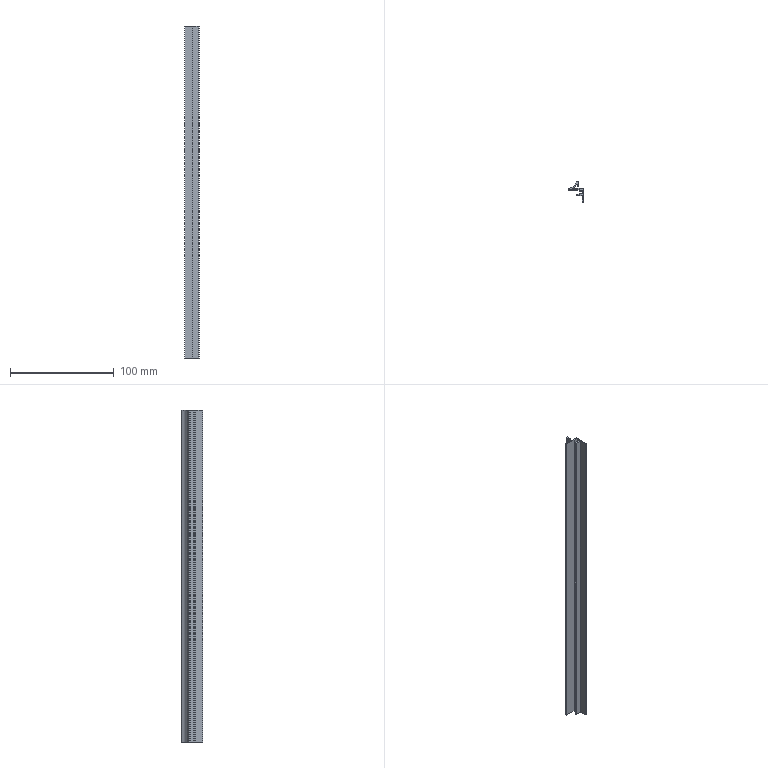Part | SolidWorks | features BaseBody 1, ICE 1, MoveFace 1 | 1 solid | 27 faces | box 14 x 20.3 x 320 mm | volume 16293 mm3 | plane 20 | cylinder 7 | commonest cylinder face diameters 0.387 x2 0.8 x2 0.4 x1 20 x1 22 x1
STEP:
#1=CARTESIAN_POINT('',(-5.304,-0.625,200.));
#2=VERTEX_POINT('',#1);
#3=CARTESIAN_POINT('',(-5.449,-0.8125,200.));
#4=VERTEX_POINT('',#3);
#5=CARTESIAN_POINT('',(-5.255,-0.8125,200.));
#6=DIRECTION('',(0.,0.,1.));
#7=DIRECTION('',(-1.,0.,0.));
#8=AXIS2_PLACEMENT_3D('',#5,#6,#7);
#9=CIRCLE('',#8,0.1937);
#10=EDGE_CURVE('',#2,#4,#9,.T.);
#11=ORIENTED_EDGE('',*,*,#10,.T.);
#12=CARTESIAN_POINT('',(-5.449,-0.8125,-120.));
#13=VERTEX_POINT('',#12);
#14=CARTESIAN_POINT('',(-5.449,-0.8125,230.));
#15=DIRECTION('',(0.,0.,-1.));
#16=VECTOR('',#15,1000.);
#17=LINE('',#14,#16);
#18=EDGE_CURVE('',#4,#13,#17,.T.);
#19=ORIENTED_EDGE('',*,*,#18,.T.);
#20=CARTESIAN_POINT('',(-5.304,-0.625,-120.));
#21=VERTEX_POINT('',#20);
#22=CARTESIAN_POINT('',(-5.255,-0.8125,-120.));
#23=DIRECTION('',(0.,0.,-1.));
#24=DIRECTION('',(1.,0.,0.));
#25=AXIS2_PLACEMENT_3D('',#22,#23,#24);
#26=CIRCLE('',#25,0.1937);
#27=EDGE_CURVE('',#13,#21,#26,.T.);
#28=ORIENTED_EDGE('',*,*,#27,.T.);
#29=CARTESIAN_POINT('',(-5.304,-0.625,230.));
#30=DIRECTION('',(0.,0.,-1.));
#31=VECTOR('',#30,1000.);
#32=LINE('',#29,#31);
#33=EDGE_CURVE('',#2,#21,#32,.T.);
#34=ORIENTED_EDGE('',*,*,#33,.F.);
#35=EDGE_LOOP('',(#11,#19,#28,#34));
#36=FACE_OUTER_BOUND('',#35,.T.);
#37=CARTESIAN_POINT('',(-5.255,-0.8125,230.));
#38=DIRECTION('',(0.,0.,-1.));
#39=DIRECTION('',(-1.,0.,0.));
#40=AXIS2_PLACEMENT_3D('',#37,#38,#39);
#41=CYLINDRICAL_SURFACE('',#40,0.1937);
#42=ADVANCED_FACE('',(#36),#41,.F.);
#43=CARTESIAN_POINT('',(5.,-1.,-120.));
#44=VERTEX_POINT('',#43);
#45=CARTESIAN_POINT('',(5.,-14.3,-120.));
#46=VERTEX_POINT('',#45);
#47=CARTESIAN_POINT('',(5.,29.623,-120.));
#48=DIRECTION('',(0.,-1.,0.));
#49=VECTOR('',#48,1000.);
#50=LINE('',#47,#49);
#51=EDGE_CURVE('',#44,#46,#50,.T.);
#52=ORIENTED_EDGE('',*,*,#51,.F.);
#53=CARTESIAN_POINT('',(5.,-1.,200.));
#54=VERTEX_POINT('',#53);
#55=CARTESIAN_POINT('',(5.,-1.,230.));
#56=DIRECTION('',(0.,0.,-1.));
#57=VECTOR('',#56,1000.);
#58=LINE('',#55,#57);
#59=EDGE_CURVE('',#54,#44,#58,.T.);
#60=ORIENTED_EDGE('',*,*,#59,.F.);
#61=CARTESIAN_POINT('',(5.,-14.3,200.));
#62=VERTEX_POINT('',#61);
#63=CARTESIAN_POINT('',(5.,-14.3,200.));
#64=DIRECTION('',(0.,1.,0.));
#65=VECTOR('',#64,1000.);
#66=LINE('',#63,#65);
#67=EDGE_CURVE('',#62,#54,#66,.T.);
#68=ORIENTED_EDGE('',*,*,#67,.F.);
#69=CARTESIAN_POINT('',(5.,-14.3,230.));
#70=DIRECTION('',(0.,0.,1.));
#71=VECTOR('',#70,1000.);
#72=LINE('',#69,#71);
#73=EDGE_CURVE('',#46,#62,#72,.T.);
#74=ORIENTED_EDGE('',*,*,#73,.F.);
#75=EDGE_LOOP('',(#52,#60,#68,#74));
#76=FACE_OUTER_BOUND('',#75,.T.);
#77=CARTESIAN_POINT('',(5.,-14.3,230.));
#78=DIRECTION('',(-1.,0.,0.));
#79=DIRECTION('',(0.,0.,1.));
#80=AXIS2_PLACEMENT_3D('',#77,#78,#79);
#81=PLANE('',#80);
#82=ADVANCED_FACE('',(#76),#81,.F.);
#83=CARTESIAN_POINT('',(-9.,-2.,-120.));
#84=VERTEX_POINT('',#83);
#85=CARTESIAN_POINT('',(-9.,-2.,200.));
#86=VERTEX_POINT('',#85);
#87=CARTESIAN_POINT('',(-9.,-2.,230.));
#88=DIRECTION('',(0.,0.,1.));
#89=VECTOR('',#88,1000.);
#90=LINE('',#87,#89);
#91=EDGE_CURVE('',#84,#86,#90,.T.);
#92=ORIENTED_EDGE('',*,*,#91,.F.);
#93=CARTESIAN_POINT('',(0.9,-2.,-120.));
#94=VERTEX_POINT('',#93);
#95=CARTESIAN_POINT('',(5.,-2.,-120.));
#96=DIRECTION('',(-1.,0.,0.));
#97=VECTOR('',#96,1000.);
#98=LINE('',#95,#97);
#99=EDGE_CURVE('',#94,#84,#98,.T.);
#100=ORIENTED_EDGE('',*,*,#99,.F.);
#101=CARTESIAN_POINT('',(0.9,-2.,200.));
#102=VERTEX_POINT('',#101);
#103=CARTESIAN_POINT('',(0.9,-2.,230.));
#104=DIRECTION('',(0.,0.,-1.));
#105=VECTOR('',#104,1000.);
#106=LINE('',#103,#105);
#107=EDGE_CURVE('',#102,#94,#106,.T.);
#108=ORIENTED_EDGE('',*,*,#107,.F.);
#109=CARTESIAN_POINT('',(5.,-2.,200.));
#110=DIRECTION('',(1.,0.,0.));
#111=VECTOR('',#110,1000.);
#112=LINE('',#109,#111);
#113=EDGE_CURVE('',#86,#102,#112,.T.);
#114=ORIENTED_EDGE('',*,*,#113,.F.);
#115=EDGE_LOOP('',(#92,#100,#108,#114));
#116=FACE_OUTER_BOUND('',#115,.T.);
#117=CARTESIAN_POINT('',(-9.,-2.,230.));
#118=DIRECTION('',(0.,1.,0.));
#119=DIRECTION('',(0.,0.,1.));
#120=AXIS2_PLACEMENT_3D('',#117,#118,#119);
#121=PLANE('',#120);
#122=ADVANCED_FACE('',(#116),#121,.F.);
#123=CARTESIAN_POINT('',(4.,-6.,200.));
#124=VERTEX_POINT('',#123);
#125=CARTESIAN_POINT('',(4.,-3.,200.));
#126=VERTEX_POINT('',#125);
#127=CARTESIAN_POINT('',(4.,29.623,200.));
#128=DIRECTION('',(0.,1.,0.));
#129=VECTOR('',#128,1000.);
#130=LINE('',#127,#129);
#131=EDGE_CURVE('',#124,#126,#130,.T.);
#132=ORIENTED_EDGE('',*,*,#131,.F.);
#133=CARTESIAN_POINT('',(1.,-6.,200.));
#134=VERTEX_POINT('',#133);
#135=CARTESIAN_POINT('',(5.,-6.,200.));
#136=DIRECTION('',(1.,0.,0.));
#137=VECTOR('',#136,1000.);
#138=LINE('',#135,#137);
#139=EDGE_CURVE('',#134,#124,#138,.T.);
#140=ORIENTED_EDGE('',*,*,#139,.F.);
#141=CARTESIAN_POINT('',(1.,-6.7,200.));
#142=VERTEX_POINT('',#141);
#143=CARTESIAN_POINT('',(1.,-6.,200.));
#144=DIRECTION('',(0.,-1.,0.));
#145=VECTOR('',#144,1000.);
#146=LINE('',#143,#145);
#147=EDGE_CURVE('',#134,#142,#146,.T.);
#148=ORIENTED_EDGE('',*,*,#147,.T.);
#149=CARTESIAN_POINT('',(-1.7,-6.7,200.));
#150=VERTEX_POINT('',#149);
#151=CARTESIAN_POINT('',(5.,-6.7,200.));
#152=DIRECTION('',(1.,0.,0.));
#153=VECTOR('',#152,1000.);
#154=LINE('',#151,#153);
#155=EDGE_CURVE('',#150,#142,#154,.T.);
#156=ORIENTED_EDGE('',*,*,#155,.F.);
#157=CARTESIAN_POINT('',(-1.7,-7.7,200.));
#158=VERTEX_POINT('',#157);
#159=CARTESIAN_POINT('',(-1.7,-6.7,200.));
#160=DIRECTION('',(0.,-1.,0.));
#161=VECTOR('',#160,1000.);
#162=LINE('',#159,#161);
#163=EDGE_CURVE('',#150,#158,#162,.T.);
#164=ORIENTED_EDGE('',*,*,#163,.T.);
#165=CARTESIAN_POINT('',(4.,-7.7,200.));
#166=VERTEX_POINT('',#165);
#167=CARTESIAN_POINT('',(5.,-7.7,200.));
#168=DIRECTION('',(-1.,0.,0.));
#169=VECTOR('',#168,1000.);
#170=LINE('',#167,#169);
#171=EDGE_CURVE('',#166,#158,#170,.T.);
#172=ORIENTED_EDGE('',*,*,#171,.F.);
#173=CARTESIAN_POINT('',(4.,-14.3,200.));
#174=VERTEX_POINT('',#173);
#175=CARTESIAN_POINT('',(4.,29.623,200.));
#176=DIRECTION('',(0.,1.,0.));
#177=VECTOR('',#176,1000.);
#178=LINE('',#175,#177);
#179=EDGE_CURVE('',#174,#166,#178,.T.);
#180=ORIENTED_EDGE('',*,*,#179,.F.);
#181=CARTESIAN_POINT('',(5.,-14.3,200.));
#182=DIRECTION('',(-1.,0.,0.));
#183=VECTOR('',#182,1000.);
#184=LINE('',#181,#183);
#185=EDGE_CURVE('',#62,#174,#184,.T.);
#186=ORIENTED_EDGE('',*,*,#185,.F.);
#187=ORIENTED_EDGE('',*,*,#67,.T.);
#188=CARTESIAN_POINT('',(-5.207,-1.,200.));
#189=VERTEX_POINT('',#188);
#190=CARTESIAN_POINT('',(5.,-1.,200.));
#191=DIRECTION('',(1.,0.,0.));
#192=VECTOR('',#191,1000.);
#193=LINE('',#190,#192);
#194=EDGE_CURVE('',#189,#54,#193,.T.);
#195=ORIENTED_EDGE('',*,*,#194,.F.);
#196=CARTESIAN_POINT('',(-5.255,-0.8125,200.));
#197=DIRECTION('',(0.,0.,1.));
#198=DIRECTION('',(-1.,0.,0.));
#199=AXIS2_PLACEMENT_3D('',#196,#197,#198);
#200=CIRCLE('',#199,0.1937);
#201=EDGE_CURVE('',#4,#189,#200,.T.);
#202=ORIENTED_EDGE('',*,*,#201,.F.);
#203=ORIENTED_EDGE('',*,*,#10,.F.);
#204=CARTESIAN_POINT('',(-1.368,3.063,200.));
#205=VERTEX_POINT('',#204);
#206=CARTESIAN_POINT('',(-10.628,9.,200.));
#207=DIRECTION('',(0.,0.,1.));
#208=DIRECTION('',(-1.,0.,0.));
#209=AXIS2_PLACEMENT_3D('',#206,#207,#208);
#210=CIRCLE('',#209,11.);
#211=EDGE_CURVE('',#2,#205,#210,.T.);
#212=ORIENTED_EDGE('',*,*,#211,.T.);
#213=CARTESIAN_POINT('',(-1.,2.955,200.));
#214=VERTEX_POINT('',#213);
#215=CARTESIAN_POINT('',(-1.2,2.955,200.));
#216=DIRECTION('',(0.,0.,1.));
#217=DIRECTION('',(-1.,0.,0.));
#218=AXIS2_PLACEMENT_3D('',#215,#216,#217);
#219=CIRCLE('',#218,0.2);
#220=EDGE_CURVE('',#214,#205,#219,.T.);
#221=ORIENTED_EDGE('',*,*,#220,.F.);
#222=CARTESIAN_POINT('',(-1.,1.5,200.));
#223=VERTEX_POINT('',#222);
#224=CARTESIAN_POINT('',(-1.,2.955,200.));
#225=DIRECTION('',(0.,1.,0.));
#226=VECTOR('',#225,1000.);
#227=LINE('',#224,#226);
#228=EDGE_CURVE('',#223,#214,#227,.T.);
#229=ORIENTED_EDGE('',*,*,#228,.F.);
#230=CARTESIAN_POINT('',(0.,1.5,200.));
#231=VERTEX_POINT('',#230);
#232=CARTESIAN_POINT('',(-1.,1.5,200.));
#233=DIRECTION('',(-1.,0.,0.));
#234=VECTOR('',#233,1000.);
#235=LINE('',#232,#234);
#236=EDGE_CURVE('',#231,#223,#235,.T.);
#237=ORIENTED_EDGE('',*,*,#236,.F.);
#238=CARTESIAN_POINT('',(0.,6.,200.));
#239=VERTEX_POINT('',#238);
#240=CARTESIAN_POINT('',(0.,1.5,200.));
#241=DIRECTION('',(0.,-1.,0.));
#242=VECTOR('',#241,1000.);
#243=LINE('',#240,#242);
#244=EDGE_CURVE('',#239,#231,#243,.T.);
#245=ORIENTED_EDGE('',*,*,#244,.F.);
#246=CARTESIAN_POINT('',(-0.8,6.,200.));
#247=VERTEX_POINT('',#246);
#248=CARTESIAN_POINT('',(0.,6.,200.));
#249=DIRECTION('',(1.,0.,0.));
#250=VECTOR('',#249,1000.);
#251=LINE('',#248,#250);
#252=EDGE_CURVE('',#247,#239,#251,.T.);
#253=ORIENTED_EDGE('',*,*,#252,.F.);
#254=CARTESIAN_POINT('',(-1.178,5.731,200.));
#255=VERTEX_POINT('',#254);
#256=CARTESIAN_POINT('',(-0.8,5.6,200.));
#257=DIRECTION('',(0.,0.,1.));
#258=DIRECTION('',(-1.,0.,0.));
#259=AXIS2_PLACEMENT_3D('',#256,#257,#258);
#260=CIRCLE('',#259,0.4);
#261=EDGE_CURVE('',#247,#255,#260,.T.);
#262=ORIENTED_EDGE('',*,*,#261,.T.);
#263=CARTESIAN_POINT('',(-8.678,-0.8077,200.));
#264=VERTEX_POINT('',#263);
#265=CARTESIAN_POINT('',(-10.628,9.,200.));
#266=DIRECTION('',(0.,0.,1.));
#267=DIRECTION('',(-1.,0.,0.));
#268=AXIS2_PLACEMENT_3D('',#265,#266,#267);
#269=CIRCLE('',#268,10.);
#270=EDGE_CURVE('',#264,#255,#269,.T.);
#271=ORIENTED_EDGE('',*,*,#270,.F.);
#272=CARTESIAN_POINT('',(-9.,-1.2,200.));
#273=VERTEX_POINT('',#272);
#274=CARTESIAN_POINT('',(-8.6,-1.2,200.));
#275=DIRECTION('',(0.,0.,1.));
#276=DIRECTION('',(-1.,0.,0.));
#277=AXIS2_PLACEMENT_3D('',#274,#275,#276);
#278=CIRCLE('',#277,0.4);
#279=EDGE_CURVE('',#264,#273,#278,.T.);
#280=ORIENTED_EDGE('',*,*,#279,.T.);
#281=CARTESIAN_POINT('',(-9.,8.,200.));
#282=DIRECTION('',(0.,-1.,0.));
#283=VECTOR('',#282,1000.);
#284=LINE('',#281,#283);
#285=EDGE_CURVE('',#273,#86,#284,.T.);
#286=ORIENTED_EDGE('',*,*,#285,.T.);
#287=ORIENTED_EDGE('',*,*,#113,.T.);
#288=CARTESIAN_POINT('',(0.9,-3.,200.));
#289=VERTEX_POINT('',#288);
#290=CARTESIAN_POINT('',(0.9,29.623,200.));
#291=DIRECTION('',(0.,1.,0.));
#292=VECTOR('',#291,1000.);
#293=LINE('',#290,#292);
#294=EDGE_CURVE('',#289,#102,#293,.T.);
#295=ORIENTED_EDGE('',*,*,#294,.F.);
#296=CARTESIAN_POINT('',(5.,-3.,200.));
#297=DIRECTION('',(-1.,0.,0.));
#298=VECTOR('',#297,1000.);
#299=LINE('',#296,#298);
#300=EDGE_CURVE('',#126,#289,#299,.T.);
#301=ORIENTED_EDGE('',*,*,#300,.F.);
#302=EDGE_LOOP('',(#132,#140,#148,#156,#164,#172,#180,#186,#187,#195,#202,#203,#212,#221,#229,#237,#245,#253,#262,#271,#280,#286,#287,#295,#301));
#303=FACE_OUTER_BOUND('',#302,.T.);
#304=CARTESIAN_POINT('',(5.,29.623,200.));
#305=DIRECTION('',(0.,0.,-1.));
#306=DIRECTION('',(-1.,0.,0.));
#307=AXIS2_PLACEMENT_3D('',#304,#305,#306);
#308=PLANE('',#307);
#309=ADVANCED_FACE('',(#303),#308,.F.);
#310=ORIENTED_EDGE('',*,*,#185,.T.);
#311=CARTESIAN_POINT('',(4.,-14.3,-120.));
#312=VERTEX_POINT('',#311);
#313=CARTESIAN_POINT('',(4.,-14.3,230.));
#314=DIRECTION('',(0.,0.,1.));
#315=VECTOR('',#314,1000.);
#316=LINE('',#313,#315);
#317=EDGE_CURVE('',#312,#174,#316,.T.);
#318=ORIENTED_EDGE('',*,*,#317,.F.);
#319=CARTESIAN_POINT('',(5.,-14.3,-120.));
#320=DIRECTION('',(-1.,0.,0.));
#321=VECTOR('',#320,1000.);
#322=LINE('',#319,#321);
#323=EDGE_CURVE('',#46,#312,#322,.T.);
#324=ORIENTED_EDGE('',*,*,#323,.F.);
#325=ORIENTED_EDGE('',*,*,#73,.T.);
#326=EDGE_LOOP('',(#310,#318,#324,#325));
#327=FACE_OUTER_BOUND('',#326,.T.);
#328=CARTESIAN_POINT('',(4.,-14.3,230.));
#329=DIRECTION('',(0.,1.,0.));
#330=DIRECTION('',(0.,0.,1.));
#331=AXIS2_PLACEMENT_3D('',#328,#329,#330);
#332=PLANE('',#331);
#333=ADVANCED_FACE('',(#327),#332,.F.);
#334=ORIENTED_EDGE('',*,*,#51,.T.);
#335=ORIENTED_EDGE('',*,*,#323,.T.);
#336=CARTESIAN_POINT('',(4.,-7.7,-120.));
#337=VERTEX_POINT('',#336);
#338=CARTESIAN_POINT('',(4.,-7.7,-120.));
#339=DIRECTION('',(0.,-1.,0.));
#340=VECTOR('',#339,1000.);
#341=LINE('',#338,#340);
#342=EDGE_CURVE('',#337,#312,#341,.T.);
#343=ORIENTED_EDGE('',*,*,#342,.F.);
#344=CARTESIAN_POINT('',(-1.7,-7.7,-120.));
#345=VERTEX_POINT('',#344);
#346=CARTESIAN_POINT('',(-1.7,-7.7,-120.));
#347=DIRECTION('',(1.,0.,0.));
#348=VECTOR('',#347,1000.);
#349=LINE('',#346,#348);
#350=EDGE_CURVE('',#345,#337,#349,.T.);
#351=ORIENTED_EDGE('',*,*,#350,.F.);
#352=CARTESIAN_POINT('',(-1.7,-6.7,-120.));
#353=VERTEX_POINT('',#352);
#354=CARTESIAN_POINT('',(-1.7,29.623,-120.));
#355=DIRECTION('',(0.,1.,0.));
#356=VECTOR('',#355,1000.);
#357=LINE('',#354,#356);
#358=EDGE_CURVE('',#345,#353,#357,.T.);
#359=ORIENTED_EDGE('',*,*,#358,.T.);
#360=CARTESIAN_POINT('',(1.,-6.7,-120.));
#361=VERTEX_POINT('',#360);
#362=CARTESIAN_POINT('',(1.,-6.7,-120.));
#363=DIRECTION('',(-1.,0.,0.));
#364=VECTOR('',#363,1000.);
#365=LINE('',#362,#364);
#366=EDGE_CURVE('',#361,#353,#365,.T.);
#367=ORIENTED_EDGE('',*,*,#366,.F.);
#368=CARTESIAN_POINT('',(1.,-6.,-120.));
#369=VERTEX_POINT('',#368);
#370=CARTESIAN_POINT('',(1.,29.623,-120.));
#371=DIRECTION('',(0.,1.,0.));
#372=VECTOR('',#371,1000.);
#373=LINE('',#370,#372);
#374=EDGE_CURVE('',#361,#369,#373,.T.);
#375=ORIENTED_EDGE('',*,*,#374,.T.);
#376=CARTESIAN_POINT('',(4.,-6.,-120.));
#377=VERTEX_POINT('',#376);
#378=CARTESIAN_POINT('',(4.,-6.,-120.));
#379=DIRECTION('',(-1.,0.,0.));
#380=VECTOR('',#379,1000.);
#381=LINE('',#378,#380);
#382=EDGE_CURVE('',#377,#369,#381,.T.);
#383=ORIENTED_EDGE('',*,*,#382,.F.);
#384=CARTESIAN_POINT('',(4.,-3.,-120.));
#385=VERTEX_POINT('',#384);
#386=CARTESIAN_POINT('',(4.,-3.,-120.));
#387=DIRECTION('',(0.,-1.,0.));
#388=VECTOR('',#387,1000.);
#389=LINE('',#386,#388);
#390=EDGE_CURVE('',#385,#377,#389,.T.);
#391=ORIENTED_EDGE('',*,*,#390,.F.);
#392=CARTESIAN_POINT('',(0.9,-3.,-120.));
#393=VERTEX_POINT('',#392);
#394=CARTESIAN_POINT('',(0.9,-3.,-120.));
#395=DIRECTION('',(1.,0.,0.));
#396=VECTOR('',#395,1000.);
#397=LINE('',#394,#396);
#398=EDGE_CURVE('',#393,#385,#397,.T.);
#399=ORIENTED_EDGE('',*,*,#398,.F.);
#400=CARTESIAN_POINT('',(0.9,-2.,-120.));
#401=DIRECTION('',(0.,-1.,0.));
#402=VECTOR('',#401,1000.);
#403=LINE('',#400,#402);
#404=EDGE_CURVE('',#94,#393,#403,.T.);
#405=ORIENTED_EDGE('',*,*,#404,.F.);
#406=ORIENTED_EDGE('',*,*,#99,.T.);
#407=CARTESIAN_POINT('',(-9.,-1.2,-120.));
#408=VERTEX_POINT('',#407);
#409=CARTESIAN_POINT('',(-9.,-1.2,-120.));
#410=DIRECTION('',(0.,-1.,0.));
#411=VECTOR('',#410,1000.);
#412=LINE('',#409,#411);
#413=EDGE_CURVE('',#408,#84,#412,.T.);
#414=ORIENTED_EDGE('',*,*,#413,.F.);
#415=CARTESIAN_POINT('',(-8.678,-0.8077,-120.));
#416=VERTEX_POINT('',#415);
#417=CARTESIAN_POINT('',(-8.6,-1.2,-120.));
#418=DIRECTION('',(0.,0.,-1.));
#419=DIRECTION('',(1.,0.,0.));
#420=AXIS2_PLACEMENT_3D('',#417,#418,#419);
#421=CIRCLE('',#420,0.4);
#422=EDGE_CURVE('',#408,#416,#421,.T.);
#423=ORIENTED_EDGE('',*,*,#422,.T.);
#424=CARTESIAN_POINT('',(-1.178,5.731,-120.));
#425=VERTEX_POINT('',#424);
#426=CARTESIAN_POINT('',(-10.628,9.,-120.));
#427=DIRECTION('',(0.,0.,-1.));
#428=DIRECTION('',(1.,0.,0.));
#429=AXIS2_PLACEMENT_3D('',#426,#427,#428);
#430=CIRCLE('',#429,10.);
#431=EDGE_CURVE('',#425,#416,#430,.T.);
#432=ORIENTED_EDGE('',*,*,#431,.F.);
#433=CARTESIAN_POINT('',(-0.8,6.,-120.));
#434=VERTEX_POINT('',#433);
#435=CARTESIAN_POINT('',(-0.8,5.6,-120.));
#436=DIRECTION('',(0.,0.,-1.));
#437=DIRECTION('',(1.,0.,0.));
#438=AXIS2_PLACEMENT_3D('',#435,#436,#437);
#439=CIRCLE('',#438,0.4);
#440=EDGE_CURVE('',#425,#434,#439,.T.);
#441=ORIENTED_EDGE('',*,*,#440,.T.);
#442=CARTESIAN_POINT('',(0.,6.,-120.));
#443=VERTEX_POINT('',#442);
#444=CARTESIAN_POINT('',(0.,6.,-120.));
#445=DIRECTION('',(-1.,0.,0.));
#446=VECTOR('',#445,1000.);
#447=LINE('',#444,#446);
#448=EDGE_CURVE('',#443,#434,#447,.T.);
#449=ORIENTED_EDGE('',*,*,#448,.F.);
#450=CARTESIAN_POINT('',(0.,1.5,-120.));
#451=VERTEX_POINT('',#450);
#452=CARTESIAN_POINT('',(0.,1.5,-120.));
#453=DIRECTION('',(0.,1.,0.));
#454=VECTOR('',#453,1000.);
#455=LINE('',#452,#454);
#456=EDGE_CURVE('',#451,#443,#455,.T.);
#457=ORIENTED_EDGE('',*,*,#456,.F.);
#458=CARTESIAN_POINT('',(-1.,1.5,-120.));
#459=VERTEX_POINT('',#458);
#460=CARTESIAN_POINT('',(-1.,1.5,-120.));
#461=DIRECTION('',(1.,0.,0.));
#462=VECTOR('',#461,1000.);
#463=LINE('',#460,#462);
#464=EDGE_CURVE('',#459,#451,#463,.T.);
#465=ORIENTED_EDGE('',*,*,#464,.F.);
#466=CARTESIAN_POINT('',(-1.,2.955,-120.));
#467=VERTEX_POINT('',#466);
#468=CARTESIAN_POINT('',(-1.,2.955,-120.));
#469=DIRECTION('',(0.,-1.,0.));
#470=VECTOR('',#469,1000.);
#471=LINE('',#468,#470);
#472=EDGE_CURVE('',#467,#459,#471,.T.);
#473=ORIENTED_EDGE('',*,*,#472,.F.);
#474=CARTESIAN_POINT('',(-1.368,3.063,-120.));
#475=VERTEX_POINT('',#474);
#476=CARTESIAN_POINT('',(-1.2,2.955,-120.));
#477=DIRECTION('',(0.,0.,-1.));
#478=DIRECTION('',(1.,0.,0.));
#479=AXIS2_PLACEMENT_3D('',#476,#477,#478);
#480=CIRCLE('',#479,0.2);
#481=EDGE_CURVE('',#475,#467,#480,.T.);
#482=ORIENTED_EDGE('',*,*,#481,.F.);
#483=CARTESIAN_POINT('',(-10.628,9.,-120.));
#484=DIRECTION('',(0.,0.,-1.));
#485=DIRECTION('',(1.,0.,0.));
#486=AXIS2_PLACEMENT_3D('',#483,#484,#485);
#487=CIRCLE('',#486,11.);
#488=EDGE_CURVE('',#475,#21,#487,.T.);
#489=ORIENTED_EDGE('',*,*,#488,.T.);
#490=ORIENTED_EDGE('',*,*,#27,.F.);
#491=CARTESIAN_POINT('',(-5.207,-1.,-120.));
#492=VERTEX_POINT('',#491);
#493=CARTESIAN_POINT('',(-5.255,-0.8125,-120.));
#494=DIRECTION('',(0.,0.,-1.));
#495=DIRECTION('',(1.,0.,0.));
#496=AXIS2_PLACEMENT_3D('',#493,#494,#495);
#497=CIRCLE('',#496,0.1937);
#498=EDGE_CURVE('',#492,#13,#497,.T.);
#499=ORIENTED_EDGE('',*,*,#498,.F.);
#500=CARTESIAN_POINT('',(5.,-1.,-120.));
#501=DIRECTION('',(-1.,0.,0.));
#502=VECTOR('',#501,1000.);
#503=LINE('',#500,#502);
#504=EDGE_CURVE('',#44,#492,#503,.T.);
#505=ORIENTED_EDGE('',*,*,#504,.F.);
#506=EDGE_LOOP('',(#334,#335,#343,#351,#359,#367,#375,#383,#391,#399,#405,#406,#414,#423,#432,#441,#449,#457,#465,#473,#482,#489,#490,#499,#505));
#507=FACE_OUTER_BOUND('',#506,.T.);
#508=CARTESIAN_POINT('',(5.,29.623,-120.));
#509=DIRECTION('',(0.,0.,1.));
#510=DIRECTION('',(1.,0.,0.));
#511=AXIS2_PLACEMENT_3D('',#508,#509,#510);
#512=PLANE('',#511);
#513=ADVANCED_FACE('',(#507),#512,.F.);
#514=ORIENTED_EDGE('',*,*,#59,.T.);
#515=ORIENTED_EDGE('',*,*,#504,.T.);
#516=CARTESIAN_POINT('',(-5.207,-1.,230.));
#517=DIRECTION('',(0.,0.,-1.));
#518=VECTOR('',#517,1000.);
#519=LINE('',#516,#518);
#520=EDGE_CURVE('',#189,#492,#519,.T.);
#521=ORIENTED_EDGE('',*,*,#520,.F.);
#522=ORIENTED_EDGE('',*,*,#194,.T.);
#523=EDGE_LOOP('',(#514,#515,#521,#522));
#524=FACE_OUTER_BOUND('',#523,.T.);
#525=CARTESIAN_POINT('',(5.,-1.,230.));
#526=DIRECTION('',(0.,-1.,0.));
#527=DIRECTION('',(0.,0.,-1.));
#528=AXIS2_PLACEMENT_3D('',#525,#526,#527);
#529=PLANE('',#528);
#530=ADVANCED_FACE('',(#524),#529,.F.);
#531=CARTESIAN_POINT('',(-9.,-1.2,230.));
#532=DIRECTION('',(0.,0.,1.));
#533=VECTOR('',#532,1000.);
#534=LINE('',#531,#533);
#535=EDGE_CURVE('',#408,#273,#534,.T.);
#536=ORIENTED_EDGE('',*,*,#535,.F.);
#537=ORIENTED_EDGE('',*,*,#413,.T.);
#538=ORIENTED_EDGE('',*,*,#91,.T.);
#539=ORIENTED_EDGE('',*,*,#285,.F.);
#540=EDGE_LOOP('',(#536,#537,#538,#539));
#541=FACE_OUTER_BOUND('',#540,.T.);
#542=CARTESIAN_POINT('',(-9.,-1.2,230.));
#543=DIRECTION('',(1.,0.,0.));
#544=DIRECTION('',(0.,0.,-1.));
#545=AXIS2_PLACEMENT_3D('',#542,#543,#544);
#546=PLANE('',#545);
#547=ADVANCED_FACE('',(#541),#546,.F.);
#548=ORIENTED_EDGE('',*,*,#294,.T.);
#549=ORIENTED_EDGE('',*,*,#107,.T.);
#550=ORIENTED_EDGE('',*,*,#404,.T.);
#551=CARTESIAN_POINT('',(0.9,-3.,230.));
#552=DIRECTION('',(0.,0.,-1.));
#553=VECTOR('',#552,1000.);
#554=LINE('',#551,#553);
#555=EDGE_CURVE('',#289,#393,#554,.T.);
#556=ORIENTED_EDGE('',*,*,#555,.F.);
#557=EDGE_LOOP('',(#548,#549,#550,#556));
#558=FACE_OUTER_BOUND('',#557,.T.);
#559=CARTESIAN_POINT('',(0.9,-2.,230.));
#560=DIRECTION('',(1.,0.,0.));
#561=DIRECTION('',(0.,0.,-1.));
#562=AXIS2_PLACEMENT_3D('',#559,#560,#561);
#563=PLANE('',#562);
#564=ADVANCED_FACE('',(#558),#563,.F.);
#565=ORIENTED_EDGE('',*,*,#300,.T.);
#566=ORIENTED_EDGE('',*,*,#555,.T.);
#567=ORIENTED_EDGE('',*,*,#398,.T.);
#568=CARTESIAN_POINT('',(4.,-3.,230.));
#569=DIRECTION('',(0.,0.,-1.));
#570=VECTOR('',#569,1000.);
#571=LINE('',#568,#570);
#572=EDGE_CURVE('',#126,#385,#571,.T.);
#573=ORIENTED_EDGE('',*,*,#572,.F.);
#574=EDGE_LOOP('',(#565,#566,#567,#573));
#575=FACE_OUTER_BOUND('',#574,.T.);
#576=CARTESIAN_POINT('',(0.9,-3.,230.));
#577=DIRECTION('',(0.,1.,0.));
#578=DIRECTION('',(0.,0.,1.));
#579=AXIS2_PLACEMENT_3D('',#576,#577,#578);
#580=PLANE('',#579);
#581=ADVANCED_FACE('',(#575),#580,.F.);
#582=ORIENTED_EDGE('',*,*,#131,.T.);
#583=ORIENTED_EDGE('',*,*,#572,.T.);
#584=ORIENTED_EDGE('',*,*,#390,.T.);
#585=CARTESIAN_POINT('',(4.,-6.,230.));
#586=DIRECTION('',(0.,0.,-1.));
#587=VECTOR('',#586,1000.);
#588=LINE('',#585,#587);
#589=EDGE_CURVE('',#124,#377,#588,.T.);
#590=ORIENTED_EDGE('',*,*,#589,.F.);
#591=EDGE_LOOP('',(#582,#583,#584,#590));
#592=FACE_OUTER_BOUND('',#591,.T.);
#593=CARTESIAN_POINT('',(4.,-3.,230.));
#594=DIRECTION('',(1.,0.,0.));
#595=DIRECTION('',(0.,0.,-1.));
#596=AXIS2_PLACEMENT_3D('',#593,#594,#595);
#597=PLANE('',#596);
#598=ADVANCED_FACE('',(#592),#597,.F.);
#599=ORIENTED_EDGE('',*,*,#139,.T.);
#600=ORIENTED_EDGE('',*,*,#589,.T.);
#601=ORIENTED_EDGE('',*,*,#382,.T.);
#602=CARTESIAN_POINT('',(1.,-6.,230.));
#603=DIRECTION('',(0.,0.,-1.));
#604=VECTOR('',#603,1000.);
#605=LINE('',#602,#604);
#606=EDGE_CURVE('',#134,#369,#605,.T.);
#607=ORIENTED_EDGE('',*,*,#606,.F.);
#608=EDGE_LOOP('',(#599,#600,#601,#607));
#609=FACE_OUTER_BOUND('',#608,.T.);
#610=CARTESIAN_POINT('',(4.,-6.,230.));
#611=DIRECTION('',(0.,-1.,0.));
#612=DIRECTION('',(0.,0.,-1.));
#613=AXIS2_PLACEMENT_3D('',#610,#611,#612);
#614=PLANE('',#613);
#615=ADVANCED_FACE('',(#609),#614,.F.);
#616=ORIENTED_EDGE('',*,*,#155,.T.);
#617=CARTESIAN_POINT('',(1.,-6.7,230.));
#618=DIRECTION('',(0.,0.,1.));
#619=VECTOR('',#618,1000.);
#620=LINE('',#617,#619);
#621=EDGE_CURVE('',#361,#142,#620,.T.);
#622=ORIENTED_EDGE('',*,*,#621,.F.);
#623=ORIENTED_EDGE('',*,*,#366,.T.);
#624=CARTESIAN_POINT('',(-1.7,-6.7,230.));
#625=DIRECTION('',(0.,0.,-1.));
#626=VECTOR('',#625,1000.);
#627=LINE('',#624,#626);
#628=EDGE_CURVE('',#150,#353,#627,.T.);
#629=ORIENTED_EDGE('',*,*,#628,.F.);
#630=EDGE_LOOP('',(#616,#622,#623,#629));
#631=FACE_OUTER_BOUND('',#630,.T.);
#632=CARTESIAN_POINT('',(1.,-6.7,230.));
#633=DIRECTION('',(0.,-1.,0.));
#634=DIRECTION('',(0.,0.,-1.));
#635=AXIS2_PLACEMENT_3D('',#632,#633,#634);
#636=PLANE('',#635);
#637=ADVANCED_FACE('',(#631),#636,.F.);
#638=ORIENTED_EDGE('',*,*,#171,.T.);
#639=CARTESIAN_POINT('',(-1.7,-7.7,230.));
#640=DIRECTION('',(0.,0.,1.));
#641=VECTOR('',#640,1000.);
#642=LINE('',#639,#641);
#643=EDGE_CURVE('',#345,#158,#642,.T.);
#644=ORIENTED_EDGE('',*,*,#643,.F.);
#645=ORIENTED_EDGE('',*,*,#350,.T.);
#646=CARTESIAN_POINT('',(4.,-7.7,230.));
#647=DIRECTION('',(0.,0.,-1.));
#648=VECTOR('',#647,1000.);
#649=LINE('',#646,#648);
#650=EDGE_CURVE('',#166,#337,#649,.T.);
#651=ORIENTED_EDGE('',*,*,#650,.F.);
#652=EDGE_LOOP('',(#638,#644,#645,#651));
#653=FACE_OUTER_BOUND('',#652,.T.);
#654=CARTESIAN_POINT('',(-1.7,-7.7,230.));
#655=DIRECTION('',(0.,1.,0.));
#656=DIRECTION('',(0.,0.,1.));
#657=AXIS2_PLACEMENT_3D('',#654,#655,#656);
#658=PLANE('',#657);
#659=ADVANCED_FACE('',(#653),#658,.F.);
#660=ORIENTED_EDGE('',*,*,#179,.T.);
#661=ORIENTED_EDGE('',*,*,#650,.T.);
#662=ORIENTED_EDGE('',*,*,#342,.T.);
#663=ORIENTED_EDGE('',*,*,#317,.T.);
#664=EDGE_LOOP('',(#660,#661,#662,#663));
#665=FACE_OUTER_BOUND('',#664,.T.);
#666=CARTESIAN_POINT('',(4.,-7.7,230.));
#667=DIRECTION('',(1.,0.,0.));
#668=DIRECTION('',(0.,0.,-1.));
#669=AXIS2_PLACEMENT_3D('',#666,#667,#668);
#670=PLANE('',#669);
#671=ADVANCED_FACE('',(#665),#670,.F.);
#672=ORIENTED_EDGE('',*,*,#18,.F.);
#673=ORIENTED_EDGE('',*,*,#201,.T.);
#674=ORIENTED_EDGE('',*,*,#520,.T.);
#675=ORIENTED_EDGE('',*,*,#498,.T.);
#676=EDGE_LOOP('',(#672,#673,#674,#675));
#677=FACE_OUTER_BOUND('',#676,.T.);
#678=CARTESIAN_POINT('',(-5.255,-0.8125,230.));
#679=DIRECTION('',(0.,0.,-1.));
#680=DIRECTION('',(-1.,0.,0.));
#681=AXIS2_PLACEMENT_3D('',#678,#679,#680);
#682=CYLINDRICAL_SURFACE('',#681,0.1937);
#683=ADVANCED_FACE('',(#677),#682,.F.);
#684=CARTESIAN_POINT('',(-1.,2.955,230.));
#685=DIRECTION('',(0.,0.,1.));
#686=VECTOR('',#685,1000.);
#687=LINE('',#684,#686);
#688=EDGE_CURVE('',#467,#214,#687,.T.);
#689=ORIENTED_EDGE('',*,*,#688,.F.);
#690=ORIENTED_EDGE('',*,*,#472,.T.);
#691=CARTESIAN_POINT('',(-1.,1.5,230.));
#692=DIRECTION('',(0.,0.,-1.));
#693=VECTOR('',#692,1000.);
#694=LINE('',#691,#693);
#695=EDGE_CURVE('',#223,#459,#694,.T.);
#696=ORIENTED_EDGE('',*,*,#695,.F.);
#697=ORIENTED_EDGE('',*,*,#228,.T.);
#698=EDGE_LOOP('',(#689,#690,#696,#697));
#699=FACE_OUTER_BOUND('',#698,.T.);
#700=CARTESIAN_POINT('',(-1.,2.955,230.));
#701=DIRECTION('',(1.,0.,0.));
#702=DIRECTION('',(0.,0.,-1.));
#703=AXIS2_PLACEMENT_3D('',#700,#701,#702);
#704=PLANE('',#703);
#705=ADVANCED_FACE('',(#699),#704,.F.);
#706=ORIENTED_EDGE('',*,*,#488,.F.);
#707=CARTESIAN_POINT('',(-1.368,3.063,230.));
#708=DIRECTION('',(0.,0.,1.));
#709=VECTOR('',#708,1000.);
#710=LINE('',#707,#709);
#711=EDGE_CURVE('',#475,#205,#710,.T.);
#712=ORIENTED_EDGE('',*,*,#711,.T.);
#713=ORIENTED_EDGE('',*,*,#211,.F.);
#714=ORIENTED_EDGE('',*,*,#33,.T.);
#715=EDGE_LOOP('',(#706,#712,#713,#714));
#716=FACE_OUTER_BOUND('',#715,.T.);
#717=CARTESIAN_POINT('',(-10.628,9.,230.));
#718=DIRECTION('',(0.,0.,-1.));
#719=DIRECTION('',(-1.,0.,0.));
#720=AXIS2_PLACEMENT_3D('',#717,#718,#719);
#721=CYLINDRICAL_SURFACE('',#720,11.);
#722=ADVANCED_FACE('',(#716),#721,.T.);
#723=CARTESIAN_POINT('',(-1.178,5.731,230.));
#724=DIRECTION('',(0.,0.,1.));
#725=VECTOR('',#724,1000.);
#726=LINE('',#723,#725);
#727=EDGE_CURVE('',#425,#255,#726,.T.);
#728=ORIENTED_EDGE('',*,*,#727,.F.);
#729=ORIENTED_EDGE('',*,*,#431,.T.);
#730=CARTESIAN_POINT('',(-8.678,-0.8077,230.));
#731=DIRECTION('',(0.,0.,-1.));
#732=VECTOR('',#731,1000.);
#733=LINE('',#730,#732);
#734=EDGE_CURVE('',#264,#416,#733,.T.);
#735=ORIENTED_EDGE('',*,*,#734,.F.);
#736=ORIENTED_EDGE('',*,*,#270,.T.);
#737=EDGE_LOOP('',(#728,#729,#735,#736));
#738=FACE_OUTER_BOUND('',#737,.T.);
#739=CARTESIAN_POINT('',(-10.628,9.,230.));
#740=DIRECTION('',(0.,0.,-1.));
#741=DIRECTION('',(-1.,0.,0.));
#742=AXIS2_PLACEMENT_3D('',#739,#740,#741);
#743=CYLINDRICAL_SURFACE('',#742,10.);
#744=ADVANCED_FACE('',(#738),#743,.F.);
#745=CARTESIAN_POINT('',(0.,1.5,230.));
#746=DIRECTION('',(0.,0.,1.));
#747=VECTOR('',#746,1000.);
#748=LINE('',#745,#747);
#749=EDGE_CURVE('',#451,#231,#748,.T.);
#750=ORIENTED_EDGE('',*,*,#749,.F.);
#751=ORIENTED_EDGE('',*,*,#456,.T.);
#752=CARTESIAN_POINT('',(0.,6.,230.));
#753=DIRECTION('',(0.,0.,-1.));
#754=VECTOR('',#753,1000.);
#755=LINE('',#752,#754);
#756=EDGE_CURVE('',#239,#443,#755,.T.);
#757=ORIENTED_EDGE('',*,*,#756,.F.);
#758=ORIENTED_EDGE('',*,*,#244,.T.);
#759=EDGE_LOOP('',(#750,#751,#757,#758));
#760=FACE_OUTER_BOUND('',#759,.T.);
#761=CARTESIAN_POINT('',(0.,1.5,230.));
#762=DIRECTION('',(-1.,0.,0.));
#763=DIRECTION('',(0.,0.,1.));
#764=AXIS2_PLACEMENT_3D('',#761,#762,#763);
#765=PLANE('',#764);
#766=ADVANCED_FACE('',(#760),#765,.F.);
#767=ORIENTED_EDGE('',*,*,#422,.F.);
#768=ORIENTED_EDGE('',*,*,#535,.T.);
#769=ORIENTED_EDGE('',*,*,#279,.F.);
#770=ORIENTED_EDGE('',*,*,#734,.T.);
#771=EDGE_LOOP('',(#767,#768,#769,#770));
#772=FACE_OUTER_BOUND('',#771,.T.);
#773=CARTESIAN_POINT('',(-8.6,-1.2,230.));
#774=DIRECTION('',(0.,0.,-1.));
#775=DIRECTION('',(-1.,0.,0.));
#776=AXIS2_PLACEMENT_3D('',#773,#774,#775);
#777=CYLINDRICAL_SURFACE('',#776,0.4);
#778=ADVANCED_FACE('',(#772),#777,.T.);
#779=ORIENTED_EDGE('',*,*,#147,.F.);
#780=ORIENTED_EDGE('',*,*,#606,.T.);
#781=ORIENTED_EDGE('',*,*,#374,.F.);
#782=ORIENTED_EDGE('',*,*,#621,.T.);
#783=EDGE_LOOP('',(#779,#780,#781,#782));
#784=FACE_OUTER_BOUND('',#783,.T.);
#785=CARTESIAN_POINT('',(1.,-6.,230.));
#786=DIRECTION('',(1.,0.,0.));
#787=DIRECTION('',(0.,0.,-1.));
#788=AXIS2_PLACEMENT_3D('',#785,#786,#787);
#789=PLANE('',#788);
#790=ADVANCED_FACE('',(#784),#789,.F.);
#791=ORIENTED_EDGE('',*,*,#163,.F.);
#792=ORIENTED_EDGE('',*,*,#628,.T.);
#793=ORIENTED_EDGE('',*,*,#358,.F.);
#794=ORIENTED_EDGE('',*,*,#643,.T.);
#795=EDGE_LOOP('',(#791,#792,#793,#794));
#796=FACE_OUTER_BOUND('',#795,.T.);
#797=CARTESIAN_POINT('',(-1.7,-6.7,230.));
#798=DIRECTION('',(1.,0.,0.));
#799=DIRECTION('',(0.,0.,-1.));
#800=AXIS2_PLACEMENT_3D('',#797,#798,#799);
#801=PLANE('',#800);
#802=ADVANCED_FACE('',(#796),#801,.F.);
#803=ORIENTED_EDGE('',*,*,#711,.F.);
#804=ORIENTED_EDGE('',*,*,#481,.T.);
#805=ORIENTED_EDGE('',*,*,#688,.T.);
#806=ORIENTED_EDGE('',*,*,#220,.T.);
#807=EDGE_LOOP('',(#803,#804,#805,#806));
#808=FACE_OUTER_BOUND('',#807,.T.);
#809=CARTESIAN_POINT('',(-1.2,2.955,230.));
#810=DIRECTION('',(0.,0.,-1.));
#811=DIRECTION('',(-1.,0.,0.));
#812=AXIS2_PLACEMENT_3D('',#809,#810,#811);
#813=CYLINDRICAL_SURFACE('',#812,0.2);
#814=ADVANCED_FACE('',(#808),#813,.F.);
#815=ORIENTED_EDGE('',*,*,#695,.T.);
#816=ORIENTED_EDGE('',*,*,#464,.T.);
#817=ORIENTED_EDGE('',*,*,#749,.T.);
#818=ORIENTED_EDGE('',*,*,#236,.T.);
#819=EDGE_LOOP('',(#815,#816,#817,#818));
#820=FACE_OUTER_BOUND('',#819,.T.);
#821=CARTESIAN_POINT('',(-1.,1.5,230.));
#822=DIRECTION('',(0.,1.,0.));
#823=DIRECTION('',(0.,0.,1.));
#824=AXIS2_PLACEMENT_3D('',#821,#822,#823);
#825=PLANE('',#824);
#826=ADVANCED_FACE('',(#820),#825,.F.);
#827=ORIENTED_EDGE('',*,*,#440,.F.);
#828=ORIENTED_EDGE('',*,*,#727,.T.);
#829=ORIENTED_EDGE('',*,*,#261,.F.);
#830=CARTESIAN_POINT('',(-0.8,6.,230.));
#831=DIRECTION('',(0.,0.,-1.));
#832=VECTOR('',#831,1000.);
#833=LINE('',#830,#832);
#834=EDGE_CURVE('',#247,#434,#833,.T.);
#835=ORIENTED_EDGE('',*,*,#834,.T.);
#836=EDGE_LOOP('',(#827,#828,#829,#835));
#837=FACE_OUTER_BOUND('',#836,.T.);
#838=CARTESIAN_POINT('',(-0.8,5.6,230.));
#839=DIRECTION('',(0.,0.,-1.));
#840=DIRECTION('',(-1.,0.,0.));
#841=AXIS2_PLACEMENT_3D('',#838,#839,#840);
#842=CYLINDRICAL_SURFACE('',#841,0.4);
#843=ADVANCED_FACE('',(#837),#842,.T.);
#844=ORIENTED_EDGE('',*,*,#756,.T.);
#845=ORIENTED_EDGE('',*,*,#448,.T.);
#846=ORIENTED_EDGE('',*,*,#834,.F.);
#847=ORIENTED_EDGE('',*,*,#252,.T.);
#848=EDGE_LOOP('',(#844,#845,#846,#847));
#849=FACE_OUTER_BOUND('',#848,.T.);
#850=CARTESIAN_POINT('',(0.,6.,230.));
#851=DIRECTION('',(0.,-1.,0.));
#852=DIRECTION('',(0.,0.,-1.));
#853=AXIS2_PLACEMENT_3D('',#850,#851,#852);
#854=PLANE('',#853);
#855=ADVANCED_FACE('',(#849),#854,.F.);
#856=CLOSED_SHELL('',(#42,#82,#122,#309,#333,#513,#530,#547,#564,#581,#598,#615,#637,#659,#671,#683,#705,#722,#744,#766,#778,#790,#802,#814,#826,#843,#855));
#857=MANIFOLD_SOLID_BREP('',#856);
#858=CARTESIAN_POINT('',(0.,0.,0.));
#859=DIRECTION('',(0.,0.,1.));
#860=DIRECTION('',(1.,0.,0.));
#861=AXIS2_PLACEMENT_3D('',#858,#859,#860);
#862=(LENGTH_UNIT()NAMED_UNIT(*)SI_UNIT(.MILLI.,.METRE.));
#863=UNCERTAINTY_MEASURE_WITH_UNIT(LENGTH_MEASURE(0.00001),#862,'','');
#864=(NAMED_UNIT(*)PLANE_ANGLE_UNIT()SI_UNIT($,.RADIAN.));
#865=(NAMED_UNIT(*)SI_UNIT($,.STERADIAN.)SOLID_ANGLE_UNIT());
#866=(GEOMETRIC_REPRESENTATION_CONTEXT(3)GLOBAL_UNCERTAINTY_ASSIGNED_CONTEXT((#863))GLOBAL_UNIT_ASSIGNED_CONTEXT((#862,#864,#865))REPRESENTATION_CONTEXT('',''));
#867=ADVANCED_BREP_SHAPE_REPRESENTATION('',(#857,#861),#866);